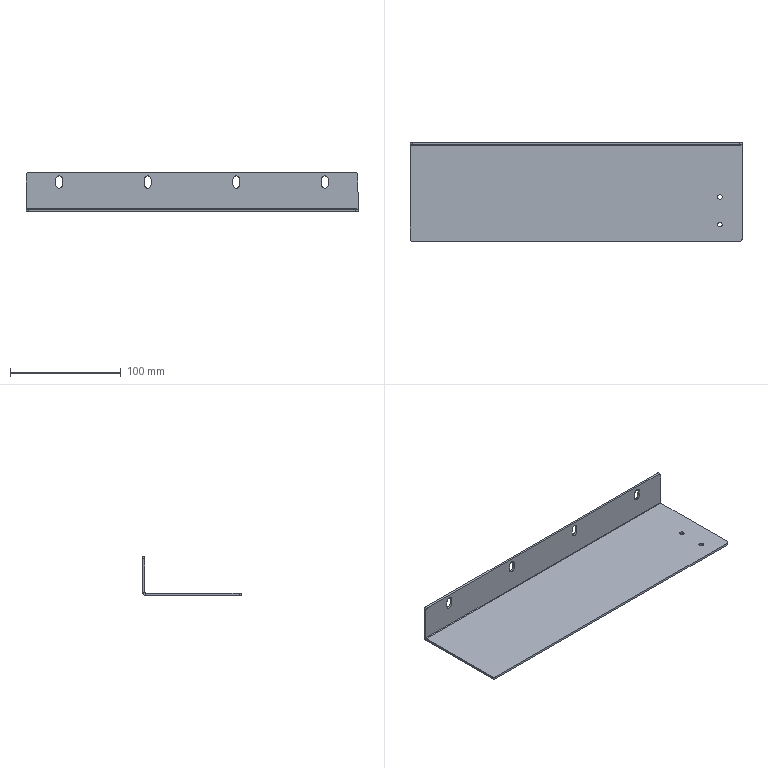Part | SolidWorks | features EdgeFlange 1, Fillet 1, FlatPattern 1, HoleWzd 1, ICE 1, LPattern 1, SMBaseFlange 1, SheetMetal 1 | 1 solid | 42 faces | box 300 x 89 x 35 mm | volume 72285 mm3 | cylinder 22 | plane 20 | commonest cylinder face diameters 6 x12 4 x4 4.2 x4 1 x1 5 x1
STEP:
#1=CARTESIAN_POINT('',(-37.,44.5,22.));
#2=VERTEX_POINT('',#1);
#3=CARTESIAN_POINT('',(-40.,44.5,19.));
#4=VERTEX_POINT('',#3);
#5=CARTESIAN_POINT('',(-40.,44.5,22.));
#6=DIRECTION('',(0.,1.,0.));
#7=DIRECTION('',(0.,0.,-1.));
#8=AXIS2_PLACEMENT_3D('',#5,#6,#7);
#9=CIRCLE('',#8,3.);
#10=EDGE_CURVE('',#2,#4,#9,.T.);
#11=ORIENTED_EDGE('',*,*,#10,.T.);
#12=CARTESIAN_POINT('',(-40.,42.5,19.));
#13=VERTEX_POINT('',#12);
#14=CARTESIAN_POINT('',(-40.,44.501,19.));
#15=DIRECTION('',(0.,-1.,0.));
#16=VECTOR('',#15,1000.);
#17=LINE('',#14,#16);
#18=EDGE_CURVE('',#4,#13,#17,.T.);
#19=ORIENTED_EDGE('',*,*,#18,.T.);
#20=CARTESIAN_POINT('',(-37.,42.5,22.));
#21=VERTEX_POINT('',#20);
#22=CARTESIAN_POINT('',(-40.,42.5,22.));
#23=DIRECTION('',(0.,-1.,0.));
#24=DIRECTION('',(0.,0.,-1.));
#25=AXIS2_PLACEMENT_3D('',#22,#23,#24);
#26=CIRCLE('',#25,3.);
#27=EDGE_CURVE('',#13,#21,#26,.T.);
#28=ORIENTED_EDGE('',*,*,#27,.T.);
#29=CARTESIAN_POINT('',(-37.,44.501,22.));
#30=DIRECTION('',(0.,-1.,0.));
#31=VECTOR('',#30,1000.);
#32=LINE('',#29,#31);
#33=EDGE_CURVE('',#2,#21,#32,.T.);
#34=ORIENTED_EDGE('',*,*,#33,.F.);
#35=EDGE_LOOP('',(#11,#19,#28,#34));
#36=FACE_OUTER_BOUND('',#35,.T.);
#37=CARTESIAN_POINT('',(-40.,44.501,22.));
#38=DIRECTION('',(0.,-1.,0.));
#39=DIRECTION('',(0.,0.,-1.));
#40=AXIS2_PLACEMENT_3D('',#37,#38,#39);
#41=CYLINDRICAL_SURFACE('',#40,3.);
#42=ADVANCED_FACE('',(#36),#41,.F.);
#43=CARTESIAN_POINT('',(-117.,44.5,22.));
#44=VERTEX_POINT('',#43);
#45=CARTESIAN_POINT('',(-120.,44.5,19.));
#46=VERTEX_POINT('',#45);
#47=CARTESIAN_POINT('',(-120.,44.5,22.));
#48=DIRECTION('',(0.,1.,0.));
#49=DIRECTION('',(0.,0.,-1.));
#50=AXIS2_PLACEMENT_3D('',#47,#48,#49);
#51=CIRCLE('',#50,3.);
#52=EDGE_CURVE('',#44,#46,#51,.T.);
#53=ORIENTED_EDGE('',*,*,#52,.T.);
#54=CARTESIAN_POINT('',(-120.,42.5,19.));
#55=VERTEX_POINT('',#54);
#56=CARTESIAN_POINT('',(-120.,44.501,19.));
#57=DIRECTION('',(0.,-1.,0.));
#58=VECTOR('',#57,1000.);
#59=LINE('',#56,#58);
#60=EDGE_CURVE('',#46,#55,#59,.T.);
#61=ORIENTED_EDGE('',*,*,#60,.T.);
#62=CARTESIAN_POINT('',(-117.,42.5,22.));
#63=VERTEX_POINT('',#62);
#64=CARTESIAN_POINT('',(-120.,42.5,22.));
#65=DIRECTION('',(0.,-1.,0.));
#66=DIRECTION('',(0.,0.,-1.));
#67=AXIS2_PLACEMENT_3D('',#64,#65,#66);
#68=CIRCLE('',#67,3.);
#69=EDGE_CURVE('',#55,#63,#68,.T.);
#70=ORIENTED_EDGE('',*,*,#69,.T.);
#71=CARTESIAN_POINT('',(-117.,44.501,22.));
#72=DIRECTION('',(0.,-1.,0.));
#73=VECTOR('',#72,1000.);
#74=LINE('',#71,#73);
#75=EDGE_CURVE('',#44,#63,#74,.T.);
#76=ORIENTED_EDGE('',*,*,#75,.F.);
#77=EDGE_LOOP('',(#53,#61,#70,#76));
#78=FACE_OUTER_BOUND('',#77,.T.);
#79=CARTESIAN_POINT('',(-120.,44.501,22.));
#80=DIRECTION('',(0.,-1.,0.));
#81=DIRECTION('',(0.,0.,-1.));
#82=AXIS2_PLACEMENT_3D('',#79,#80,#81);
#83=CYLINDRICAL_SURFACE('',#82,3.);
#84=ADVANCED_FACE('',(#78),#83,.F.);
#85=CARTESIAN_POINT('',(127.9,-29.5,-2.));
#86=VERTEX_POINT('',#85);
#87=CARTESIAN_POINT('',(132.1,-29.5,-2.));
#88=VERTEX_POINT('',#87);
#89=CARTESIAN_POINT('',(130.,-29.5,-2.));
#90=DIRECTION('',(0.,0.,1.));
#91=DIRECTION('',(1.,0.,0.));
#92=AXIS2_PLACEMENT_3D('',#89,#90,#91);
#93=CIRCLE('',#92,2.1);
#94=EDGE_CURVE('',#86,#88,#93,.T.);
#95=ORIENTED_EDGE('',*,*,#94,.F.);
#96=CARTESIAN_POINT('',(127.9,-29.5,0.));
#97=VERTEX_POINT('',#96);
#98=CARTESIAN_POINT('',(127.9,-29.5,0.));
#99=DIRECTION('',(0.,0.,1.));
#100=VECTOR('',#99,1000.);
#101=LINE('',#98,#100);
#102=EDGE_CURVE('',#86,#97,#101,.T.);
#103=ORIENTED_EDGE('',*,*,#102,.T.);
#104=CARTESIAN_POINT('',(132.1,-29.5,0.));
#105=VERTEX_POINT('',#104);
#106=CARTESIAN_POINT('',(130.,-29.5,0.));
#107=DIRECTION('',(0.,0.,1.));
#108=DIRECTION('',(1.,0.,0.));
#109=AXIS2_PLACEMENT_3D('',#106,#107,#108);
#110=CIRCLE('',#109,2.1);
#111=EDGE_CURVE('',#97,#105,#110,.T.);
#112=ORIENTED_EDGE('',*,*,#111,.T.);
#113=CARTESIAN_POINT('',(132.1,-29.5,0.));
#114=DIRECTION('',(0.,0.,1.));
#115=VECTOR('',#114,1000.);
#116=LINE('',#113,#115);
#117=EDGE_CURVE('',#88,#105,#116,.T.);
#118=ORIENTED_EDGE('',*,*,#117,.F.);
#119=EDGE_LOOP('',(#95,#103,#112,#118));
#120=FACE_OUTER_BOUND('',#119,.T.);
#121=CARTESIAN_POINT('',(130.,-29.5,0.));
#122=DIRECTION('',(0.,0.,1.));
#123=DIRECTION('',(1.,0.,0.));
#124=AXIS2_PLACEMENT_3D('',#121,#122,#123);
#125=CYLINDRICAL_SURFACE('',#124,2.1);
#126=ADVANCED_FACE('',(#120),#125,.F.);
#127=CARTESIAN_POINT('',(127.9,-4.5,-2.));
#128=VERTEX_POINT('',#127);
#129=CARTESIAN_POINT('',(132.1,-4.5,-2.));
#130=VERTEX_POINT('',#129);
#131=CARTESIAN_POINT('',(130.,-4.5,-2.));
#132=DIRECTION('',(0.,0.,1.));
#133=DIRECTION('',(1.,0.,0.));
#134=AXIS2_PLACEMENT_3D('',#131,#132,#133);
#135=CIRCLE('',#134,2.1);
#136=EDGE_CURVE('',#128,#130,#135,.T.);
#137=ORIENTED_EDGE('',*,*,#136,.F.);
#138=CARTESIAN_POINT('',(127.9,-4.5,0.));
#139=VERTEX_POINT('',#138);
#140=CARTESIAN_POINT('',(127.9,-4.5,0.));
#141=DIRECTION('',(0.,0.,1.));
#142=VECTOR('',#141,1000.);
#143=LINE('',#140,#142);
#144=EDGE_CURVE('',#128,#139,#143,.T.);
#145=ORIENTED_EDGE('',*,*,#144,.T.);
#146=CARTESIAN_POINT('',(132.1,-4.5,0.));
#147=VERTEX_POINT('',#146);
#148=CARTESIAN_POINT('',(130.,-4.5,0.));
#149=DIRECTION('',(0.,0.,1.));
#150=DIRECTION('',(1.,0.,0.));
#151=AXIS2_PLACEMENT_3D('',#148,#149,#150);
#152=CIRCLE('',#151,2.1);
#153=EDGE_CURVE('',#139,#147,#152,.T.);
#154=ORIENTED_EDGE('',*,*,#153,.T.);
#155=CARTESIAN_POINT('',(132.1,-4.5,0.));
#156=DIRECTION('',(0.,0.,1.));
#157=VECTOR('',#156,1000.);
#158=LINE('',#155,#157);
#159=EDGE_CURVE('',#130,#147,#158,.T.);
#160=ORIENTED_EDGE('',*,*,#159,.F.);
#161=EDGE_LOOP('',(#137,#145,#154,#160));
#162=FACE_OUTER_BOUND('',#161,.T.);
#163=CARTESIAN_POINT('',(130.,-4.5,0.));
#164=DIRECTION('',(0.,0.,1.));
#165=DIRECTION('',(1.,0.,0.));
#166=AXIS2_PLACEMENT_3D('',#163,#164,#165);
#167=CYLINDRICAL_SURFACE('',#166,2.1);
#168=ADVANCED_FACE('',(#162),#167,.F.);
#169=CARTESIAN_POINT('',(43.,44.5,22.));
#170=VERTEX_POINT('',#169);
#171=CARTESIAN_POINT('',(40.,44.5,19.));
#172=VERTEX_POINT('',#171);
#173=CARTESIAN_POINT('',(40.,44.5,22.));
#174=DIRECTION('',(0.,1.,0.));
#175=DIRECTION('',(0.,0.,-1.));
#176=AXIS2_PLACEMENT_3D('',#173,#174,#175);
#177=CIRCLE('',#176,3.);
#178=EDGE_CURVE('',#170,#172,#177,.T.);
#179=ORIENTED_EDGE('',*,*,#178,.T.);
#180=CARTESIAN_POINT('',(40.,42.5,19.));
#181=VERTEX_POINT('',#180);
#182=CARTESIAN_POINT('',(40.,44.501,19.));
#183=DIRECTION('',(0.,-1.,0.));
#184=VECTOR('',#183,1000.);
#185=LINE('',#182,#184);
#186=EDGE_CURVE('',#172,#181,#185,.T.);
#187=ORIENTED_EDGE('',*,*,#186,.T.);
#188=CARTESIAN_POINT('',(43.,42.5,22.));
#189=VERTEX_POINT('',#188);
#190=CARTESIAN_POINT('',(40.,42.5,22.));
#191=DIRECTION('',(0.,-1.,0.));
#192=DIRECTION('',(0.,0.,-1.));
#193=AXIS2_PLACEMENT_3D('',#190,#191,#192);
#194=CIRCLE('',#193,3.);
#195=EDGE_CURVE('',#181,#189,#194,.T.);
#196=ORIENTED_EDGE('',*,*,#195,.T.);
#197=CARTESIAN_POINT('',(43.,44.501,22.));
#198=DIRECTION('',(0.,-1.,0.));
#199=VECTOR('',#198,1000.);
#200=LINE('',#197,#199);
#201=EDGE_CURVE('',#170,#189,#200,.T.);
#202=ORIENTED_EDGE('',*,*,#201,.F.);
#203=EDGE_LOOP('',(#179,#187,#196,#202));
#204=FACE_OUTER_BOUND('',#203,.T.);
#205=CARTESIAN_POINT('',(40.,44.501,22.));
#206=DIRECTION('',(0.,-1.,0.));
#207=DIRECTION('',(0.,0.,-1.));
#208=AXIS2_PLACEMENT_3D('',#205,#206,#207);
#209=CYLINDRICAL_SURFACE('',#208,3.);
#210=ADVANCED_FACE('',(#204),#209,.F.);
#211=CARTESIAN_POINT('',(123.,44.5,22.));
#212=VERTEX_POINT('',#211);
#213=CARTESIAN_POINT('',(120.,44.5,19.));
#214=VERTEX_POINT('',#213);
#215=CARTESIAN_POINT('',(120.,44.5,22.));
#216=DIRECTION('',(0.,1.,0.));
#217=DIRECTION('',(0.,0.,-1.));
#218=AXIS2_PLACEMENT_3D('',#215,#216,#217);
#219=CIRCLE('',#218,3.);
#220=EDGE_CURVE('',#212,#214,#219,.T.);
#221=ORIENTED_EDGE('',*,*,#220,.T.);
#222=CARTESIAN_POINT('',(120.,42.5,19.));
#223=VERTEX_POINT('',#222);
#224=CARTESIAN_POINT('',(120.,44.501,19.));
#225=DIRECTION('',(0.,-1.,0.));
#226=VECTOR('',#225,1000.);
#227=LINE('',#224,#226);
#228=EDGE_CURVE('',#214,#223,#227,.T.);
#229=ORIENTED_EDGE('',*,*,#228,.T.);
#230=CARTESIAN_POINT('',(123.,42.5,22.));
#231=VERTEX_POINT('',#230);
#232=CARTESIAN_POINT('',(120.,42.5,22.));
#233=DIRECTION('',(0.,-1.,0.));
#234=DIRECTION('',(0.,0.,-1.));
#235=AXIS2_PLACEMENT_3D('',#232,#233,#234);
#236=CIRCLE('',#235,3.);
#237=EDGE_CURVE('',#223,#231,#236,.T.);
#238=ORIENTED_EDGE('',*,*,#237,.T.);
#239=CARTESIAN_POINT('',(123.,44.501,22.));
#240=DIRECTION('',(0.,-1.,0.));
#241=VECTOR('',#240,1000.);
#242=LINE('',#239,#241);
#243=EDGE_CURVE('',#212,#231,#242,.T.);
#244=ORIENTED_EDGE('',*,*,#243,.F.);
#245=EDGE_LOOP('',(#221,#229,#238,#244));
#246=FACE_OUTER_BOUND('',#245,.T.);
#247=CARTESIAN_POINT('',(120.,44.501,22.));
#248=DIRECTION('',(0.,-1.,0.));
#249=DIRECTION('',(0.,0.,-1.));
#250=AXIS2_PLACEMENT_3D('',#247,#248,#249);
#251=CYLINDRICAL_SURFACE('',#250,3.);
#252=ADVANCED_FACE('',(#246),#251,.F.);
#253=CARTESIAN_POINT('',(117.,44.5,22.));
#254=VERTEX_POINT('',#253);
#255=CARTESIAN_POINT('',(117.,44.5,27.));
#256=VERTEX_POINT('',#255);
#257=CARTESIAN_POINT('',(117.,44.5,27.));
#258=DIRECTION('',(0.,0.,1.));
#259=VECTOR('',#258,1000.);
#260=LINE('',#257,#259);
#261=EDGE_CURVE('',#254,#256,#260,.T.);
#262=ORIENTED_EDGE('',*,*,#261,.T.);
#263=CARTESIAN_POINT('',(117.,42.5,27.));
#264=VERTEX_POINT('',#263);
#265=CARTESIAN_POINT('',(117.,44.501,27.));
#266=DIRECTION('',(0.,-1.,0.));
#267=VECTOR('',#266,1000.);
#268=LINE('',#265,#267);
#269=EDGE_CURVE('',#256,#264,#268,.T.);
#270=ORIENTED_EDGE('',*,*,#269,.T.);
#271=CARTESIAN_POINT('',(117.,42.5,22.));
#272=VERTEX_POINT('',#271);
#273=CARTESIAN_POINT('',(117.,42.5,27.));
#274=DIRECTION('',(0.,0.,-1.));
#275=VECTOR('',#274,1000.);
#276=LINE('',#273,#275);
#277=EDGE_CURVE('',#264,#272,#276,.T.);
#278=ORIENTED_EDGE('',*,*,#277,.T.);
#279=CARTESIAN_POINT('',(117.,44.501,22.));
#280=DIRECTION('',(0.,-1.,0.));
#281=VECTOR('',#280,1000.);
#282=LINE('',#279,#281);
#283=EDGE_CURVE('',#254,#272,#282,.T.);
#284=ORIENTED_EDGE('',*,*,#283,.F.);
#285=EDGE_LOOP('',(#262,#270,#278,#284));
#286=FACE_OUTER_BOUND('',#285,.T.);
#287=CARTESIAN_POINT('',(117.,44.501,27.));
#288=DIRECTION('',(-1.,0.,0.));
#289=DIRECTION('',(0.,-1.,0.));
#290=AXIS2_PLACEMENT_3D('',#287,#288,#289);
#291=PLANE('',#290);
#292=ADVANCED_FACE('',(#286),#291,.F.);
#293=ORIENTED_EDGE('',*,*,#228,.F.);
#294=CARTESIAN_POINT('',(120.,44.5,22.));
#295=DIRECTION('',(0.,1.,0.));
#296=DIRECTION('',(0.,0.,-1.));
#297=AXIS2_PLACEMENT_3D('',#294,#295,#296);
#298=CIRCLE('',#297,3.);
#299=EDGE_CURVE('',#214,#254,#298,.T.);
#300=ORIENTED_EDGE('',*,*,#299,.T.);
#301=ORIENTED_EDGE('',*,*,#283,.T.);
#302=CARTESIAN_POINT('',(120.,42.5,22.));
#303=DIRECTION('',(0.,-1.,0.));
#304=DIRECTION('',(0.,0.,-1.));
#305=AXIS2_PLACEMENT_3D('',#302,#303,#304);
#306=CIRCLE('',#305,3.);
#307=EDGE_CURVE('',#272,#223,#306,.T.);
#308=ORIENTED_EDGE('',*,*,#307,.T.);
#309=EDGE_LOOP('',(#293,#300,#301,#308));
#310=FACE_OUTER_BOUND('',#309,.T.);
#311=CARTESIAN_POINT('',(120.,44.501,22.));
#312=DIRECTION('',(0.,-1.,0.));
#313=DIRECTION('',(0.,0.,-1.));
#314=AXIS2_PLACEMENT_3D('',#311,#312,#313);
#315=CYLINDRICAL_SURFACE('',#314,3.);
#316=ADVANCED_FACE('',(#310),#315,.F.);
#317=CARTESIAN_POINT('',(123.,44.5,27.));
#318=VERTEX_POINT('',#317);
#319=CARTESIAN_POINT('',(123.,44.5,27.));
#320=DIRECTION('',(0.,0.,-1.));
#321=VECTOR('',#320,1000.);
#322=LINE('',#319,#321);
#323=EDGE_CURVE('',#318,#212,#322,.T.);
#324=ORIENTED_EDGE('',*,*,#323,.T.);
#325=ORIENTED_EDGE('',*,*,#243,.T.);
#326=CARTESIAN_POINT('',(123.,42.5,27.));
#327=VERTEX_POINT('',#326);
#328=CARTESIAN_POINT('',(123.,42.5,27.));
#329=DIRECTION('',(0.,0.,1.));
#330=VECTOR('',#329,1000.);
#331=LINE('',#328,#330);
#332=EDGE_CURVE('',#231,#327,#331,.T.);
#333=ORIENTED_EDGE('',*,*,#332,.T.);
#334=CARTESIAN_POINT('',(123.,44.501,27.));
#335=DIRECTION('',(0.,-1.,0.));
#336=VECTOR('',#335,1000.);
#337=LINE('',#334,#336);
#338=EDGE_CURVE('',#318,#327,#337,.T.);
#339=ORIENTED_EDGE('',*,*,#338,.F.);
#340=EDGE_LOOP('',(#324,#325,#333,#339));
#341=FACE_OUTER_BOUND('',#340,.T.);
#342=CARTESIAN_POINT('',(123.,44.501,27.));
#343=DIRECTION('',(1.,0.,0.));
#344=DIRECTION('',(0.,1.,0.));
#345=AXIS2_PLACEMENT_3D('',#342,#343,#344);
#346=PLANE('',#345);
#347=ADVANCED_FACE('',(#341),#346,.F.);
#348=CARTESIAN_POINT('',(120.,44.5,27.));
#349=DIRECTION('',(0.,1.,0.));
#350=DIRECTION('',(0.,0.,-1.));
#351=AXIS2_PLACEMENT_3D('',#348,#349,#350);
#352=CIRCLE('',#351,3.);
#353=EDGE_CURVE('',#256,#318,#352,.T.);
#354=ORIENTED_EDGE('',*,*,#353,.T.);
#355=ORIENTED_EDGE('',*,*,#338,.T.);
#356=CARTESIAN_POINT('',(120.,42.5,27.));
#357=DIRECTION('',(0.,-1.,0.));
#358=DIRECTION('',(0.,0.,-1.));
#359=AXIS2_PLACEMENT_3D('',#356,#357,#358);
#360=CIRCLE('',#359,3.);
#361=EDGE_CURVE('',#327,#264,#360,.T.);
#362=ORIENTED_EDGE('',*,*,#361,.T.);
#363=ORIENTED_EDGE('',*,*,#269,.F.);
#364=EDGE_LOOP('',(#354,#355,#362,#363));
#365=FACE_OUTER_BOUND('',#364,.T.);
#366=CARTESIAN_POINT('',(120.,44.501,27.));
#367=DIRECTION('',(0.,-1.,0.));
#368=DIRECTION('',(0.,0.,-1.));
#369=AXIS2_PLACEMENT_3D('',#366,#367,#368);
#370=CYLINDRICAL_SURFACE('',#369,3.);
#371=ADVANCED_FACE('',(#365),#370,.F.);
#372=CARTESIAN_POINT('',(37.,44.5,22.));
#373=VERTEX_POINT('',#372);
#374=CARTESIAN_POINT('',(37.,44.5,27.));
#375=VERTEX_POINT('',#374);
#376=CARTESIAN_POINT('',(37.,44.5,27.));
#377=DIRECTION('',(0.,0.,1.));
#378=VECTOR('',#377,1000.);
#379=LINE('',#376,#378);
#380=EDGE_CURVE('',#373,#375,#379,.T.);
#381=ORIENTED_EDGE('',*,*,#380,.T.);
#382=CARTESIAN_POINT('',(37.,42.5,27.));
#383=VERTEX_POINT('',#382);
#384=CARTESIAN_POINT('',(37.,44.501,27.));
#385=DIRECTION('',(0.,-1.,0.));
#386=VECTOR('',#385,1000.);
#387=LINE('',#384,#386);
#388=EDGE_CURVE('',#375,#383,#387,.T.);
#389=ORIENTED_EDGE('',*,*,#388,.T.);
#390=CARTESIAN_POINT('',(37.,42.5,22.));
#391=VERTEX_POINT('',#390);
#392=CARTESIAN_POINT('',(37.,42.5,27.));
#393=DIRECTION('',(0.,0.,-1.));
#394=VECTOR('',#393,1000.);
#395=LINE('',#392,#394);
#396=EDGE_CURVE('',#383,#391,#395,.T.);
#397=ORIENTED_EDGE('',*,*,#396,.T.);
#398=CARTESIAN_POINT('',(37.,44.501,22.));
#399=DIRECTION('',(0.,-1.,0.));
#400=VECTOR('',#399,1000.);
#401=LINE('',#398,#400);
#402=EDGE_CURVE('',#373,#391,#401,.T.);
#403=ORIENTED_EDGE('',*,*,#402,.F.);
#404=EDGE_LOOP('',(#381,#389,#397,#403));
#405=FACE_OUTER_BOUND('',#404,.T.);
#406=CARTESIAN_POINT('',(37.,44.501,27.));
#407=DIRECTION('',(-1.,0.,0.));
#408=DIRECTION('',(0.,-1.,0.));
#409=AXIS2_PLACEMENT_3D('',#406,#407,#408);
#410=PLANE('',#409);
#411=ADVANCED_FACE('',(#405),#410,.F.);
#412=ORIENTED_EDGE('',*,*,#186,.F.);
#413=CARTESIAN_POINT('',(40.,44.5,22.));
#414=DIRECTION('',(0.,1.,0.));
#415=DIRECTION('',(0.,0.,-1.));
#416=AXIS2_PLACEMENT_3D('',#413,#414,#415);
#417=CIRCLE('',#416,3.);
#418=EDGE_CURVE('',#172,#373,#417,.T.);
#419=ORIENTED_EDGE('',*,*,#418,.T.);
#420=ORIENTED_EDGE('',*,*,#402,.T.);
#421=CARTESIAN_POINT('',(40.,42.5,22.));
#422=DIRECTION('',(0.,-1.,0.));
#423=DIRECTION('',(0.,0.,-1.));
#424=AXIS2_PLACEMENT_3D('',#421,#422,#423);
#425=CIRCLE('',#424,3.);
#426=EDGE_CURVE('',#391,#181,#425,.T.);
#427=ORIENTED_EDGE('',*,*,#426,.T.);
#428=EDGE_LOOP('',(#412,#419,#420,#427));
#429=FACE_OUTER_BOUND('',#428,.T.);
#430=CARTESIAN_POINT('',(40.,44.501,22.));
#431=DIRECTION('',(0.,-1.,0.));
#432=DIRECTION('',(0.,0.,-1.));
#433=AXIS2_PLACEMENT_3D('',#430,#431,#432);
#434=CYLINDRICAL_SURFACE('',#433,3.);
#435=ADVANCED_FACE('',(#429),#434,.F.);
#436=CARTESIAN_POINT('',(43.,44.5,27.));
#437=VERTEX_POINT('',#436);
#438=CARTESIAN_POINT('',(43.,44.5,27.));
#439=DIRECTION('',(0.,0.,-1.));
#440=VECTOR('',#439,1000.);
#441=LINE('',#438,#440);
#442=EDGE_CURVE('',#437,#170,#441,.T.);
#443=ORIENTED_EDGE('',*,*,#442,.T.);
#444=ORIENTED_EDGE('',*,*,#201,.T.);
#445=CARTESIAN_POINT('',(43.,42.5,27.));
#446=VERTEX_POINT('',#445);
#447=CARTESIAN_POINT('',(43.,42.5,27.));
#448=DIRECTION('',(0.,0.,1.));
#449=VECTOR('',#448,1000.);
#450=LINE('',#447,#449);
#451=EDGE_CURVE('',#189,#446,#450,.T.);
#452=ORIENTED_EDGE('',*,*,#451,.T.);
#453=CARTESIAN_POINT('',(43.,44.501,27.));
#454=DIRECTION('',(0.,-1.,0.));
#455=VECTOR('',#454,1000.);
#456=LINE('',#453,#455);
#457=EDGE_CURVE('',#437,#446,#456,.T.);
#458=ORIENTED_EDGE('',*,*,#457,.F.);
#459=EDGE_LOOP('',(#443,#444,#452,#458));
#460=FACE_OUTER_BOUND('',#459,.T.);
#461=CARTESIAN_POINT('',(43.,44.501,27.));
#462=DIRECTION('',(1.,0.,0.));
#463=DIRECTION('',(0.,1.,0.));
#464=AXIS2_PLACEMENT_3D('',#461,#462,#463);
#465=PLANE('',#464);
#466=ADVANCED_FACE('',(#460),#465,.F.);
#467=CARTESIAN_POINT('',(40.,44.5,27.));
#468=DIRECTION('',(0.,1.,0.));
#469=DIRECTION('',(0.,0.,-1.));
#470=AXIS2_PLACEMENT_3D('',#467,#468,#469);
#471=CIRCLE('',#470,3.);
#472=EDGE_CURVE('',#375,#437,#471,.T.);
#473=ORIENTED_EDGE('',*,*,#472,.T.);
#474=ORIENTED_EDGE('',*,*,#457,.T.);
#475=CARTESIAN_POINT('',(40.,42.5,27.));
#476=DIRECTION('',(0.,-1.,0.));
#477=DIRECTION('',(0.,0.,-1.));
#478=AXIS2_PLACEMENT_3D('',#475,#476,#477);
#479=CIRCLE('',#478,3.);
#480=EDGE_CURVE('',#446,#383,#479,.T.);
#481=ORIENTED_EDGE('',*,*,#480,.T.);
#482=ORIENTED_EDGE('',*,*,#388,.F.);
#483=EDGE_LOOP('',(#473,#474,#481,#482));
#484=FACE_OUTER_BOUND('',#483,.T.);
#485=CARTESIAN_POINT('',(40.,44.501,27.));
#486=DIRECTION('',(0.,-1.,0.));
#487=DIRECTION('',(0.,0.,-1.));
#488=AXIS2_PLACEMENT_3D('',#485,#486,#487);
#489=CYLINDRICAL_SURFACE('',#488,3.);
#490=ADVANCED_FACE('',(#484),#489,.F.);
#491=CARTESIAN_POINT('',(-150.,42.,-2.));
#492=VERTEX_POINT('',#491);
#493=CARTESIAN_POINT('',(-150.,-42.5,-2.));
#494=VERTEX_POINT('',#493);
#495=CARTESIAN_POINT('',(-150.,-44.5,-2.));
#496=DIRECTION('',(0.,-1.,0.));
#497=VECTOR('',#496,1000.);
#498=LINE('',#495,#497);
#499=EDGE_CURVE('',#492,#494,#498,.T.);
#500=ORIENTED_EDGE('',*,*,#499,.T.);
#501=CARTESIAN_POINT('',(-150.,-42.5,0.));
#502=VERTEX_POINT('',#501);
#503=CARTESIAN_POINT('',(-150.,-42.5,-2.));
#504=DIRECTION('',(0.,0.,1.));
#505=VECTOR('',#504,1000.);
#506=LINE('',#503,#505);
#507=EDGE_CURVE('',#494,#502,#506,.T.);
#508=ORIENTED_EDGE('',*,*,#507,.T.);
#509=CARTESIAN_POINT('',(-150.,42.,0.));
#510=VERTEX_POINT('',#509);
#511=CARTESIAN_POINT('',(-150.,-44.5,0.));
#512=DIRECTION('',(0.,-1.,0.));
#513=VECTOR('',#512,1000.);
#514=LINE('',#511,#513);
#515=EDGE_CURVE('',#510,#502,#514,.T.);
#516=ORIENTED_EDGE('',*,*,#515,.F.);
#517=CARTESIAN_POINT('',(-150.,42.,0.));
#518=DIRECTION('',(0.,0.,-1.));
#519=VECTOR('',#518,1000.);
#520=LINE('',#517,#519);
#521=EDGE_CURVE('',#510,#492,#520,.T.);
#522=ORIENTED_EDGE('',*,*,#521,.T.);
#523=EDGE_LOOP('',(#500,#508,#516,#522));
#524=FACE_OUTER_BOUND('',#523,.T.);
#525=CARTESIAN_POINT('',(-150.,-44.5,-2.));
#526=DIRECTION('',(-1.,0.,0.));
#527=DIRECTION('',(0.,0.,1.));
#528=AXIS2_PLACEMENT_3D('',#525,#526,#527);
#529=PLANE('',#528);
#530=ADVANCED_FACE('',(#524),#529,.T.);
#531=CARTESIAN_POINT('',(130.,-29.5,-2.));
#532=DIRECTION('',(0.,0.,1.));
#533=DIRECTION('',(1.,0.,0.));
#534=AXIS2_PLACEMENT_3D('',#531,#532,#533);
#535=CIRCLE('',#534,2.1);
#536=EDGE_CURVE('',#88,#86,#535,.T.);
#537=ORIENTED_EDGE('',*,*,#536,.T.);
#538=ORIENTED_EDGE('',*,*,#94,.T.);
#539=EDGE_LOOP('',(#537,#538));
#540=FACE_BOUND('',#539,.T.);
#541=CARTESIAN_POINT('',(130.,-4.5,-2.));
#542=DIRECTION('',(0.,0.,1.));
#543=DIRECTION('',(1.,0.,0.));
#544=AXIS2_PLACEMENT_3D('',#541,#542,#543);
#545=CIRCLE('',#544,2.1);
#546=EDGE_CURVE('',#130,#128,#545,.T.);
#547=ORIENTED_EDGE('',*,*,#546,.T.);
#548=ORIENTED_EDGE('',*,*,#136,.T.);
#549=EDGE_LOOP('',(#547,#548));
#550=FACE_BOUND('',#549,.T.);
#551=CARTESIAN_POINT('',(-148.,-44.5,-2.));
#552=VERTEX_POINT('',#551);
#553=CARTESIAN_POINT('',(148.,-44.5,-2.));
#554=VERTEX_POINT('',#553);
#555=CARTESIAN_POINT('',(150.,-44.5,-2.));
#556=DIRECTION('',(1.,0.,0.));
#557=VECTOR('',#556,1000.);
#558=LINE('',#555,#557);
#559=EDGE_CURVE('',#552,#554,#558,.T.);
#560=ORIENTED_EDGE('',*,*,#559,.F.);
#561=CARTESIAN_POINT('',(-148.,-42.5,-2.));
#562=DIRECTION('',(0.,0.,-1.));
#563=DIRECTION('',(1.,0.,0.));
#564=AXIS2_PLACEMENT_3D('',#561,#562,#563);
#565=CIRCLE('',#564,2.);
#566=EDGE_CURVE('',#552,#494,#565,.T.);
#567=ORIENTED_EDGE('',*,*,#566,.T.);
#568=ORIENTED_EDGE('',*,*,#499,.F.);
#569=CARTESIAN_POINT('',(150.,42.,-2.));
#570=VERTEX_POINT('',#569);
#571=CARTESIAN_POINT('',(-150.,42.,-2.));
#572=DIRECTION('',(1.,0.,0.));
#573=VECTOR('',#572,1000.);
#574=LINE('',#571,#573);
#575=EDGE_CURVE('',#492,#570,#574,.T.);
#576=ORIENTED_EDGE('',*,*,#575,.T.);
#577=CARTESIAN_POINT('',(150.,-42.5,-2.));
#578=VERTEX_POINT('',#577);
#579=CARTESIAN_POINT('',(150.,-44.5,-2.));
#580=DIRECTION('',(0.,1.,0.));
#581=VECTOR('',#580,1000.);
#582=LINE('',#579,#581);
#583=EDGE_CURVE('',#578,#570,#582,.T.);
#584=ORIENTED_EDGE('',*,*,#583,.F.);
#585=CARTESIAN_POINT('',(148.,-42.5,-2.));
#586=DIRECTION('',(0.,0.,-1.));
#587=DIRECTION('',(1.,0.,0.));
#588=AXIS2_PLACEMENT_3D('',#585,#586,#587);
#589=CIRCLE('',#588,2.);
#590=EDGE_CURVE('',#578,#554,#589,.T.);
#591=ORIENTED_EDGE('',*,*,#590,.T.);
#592=EDGE_LOOP('',(#560,#567,#568,#576,#584,#591));
#593=FACE_OUTER_BOUND('',#592,.T.);
#594=CARTESIAN_POINT('',(0.,0.,-2.));
#595=DIRECTION('',(0.,0.,1.));
#596=DIRECTION('',(1.,0.,0.));
#597=AXIS2_PLACEMENT_3D('',#594,#595,#596);
#598=PLANE('',#597);
#599=ADVANCED_FACE('',(#540,#550,#593),#598,.F.);
#600=CARTESIAN_POINT('',(130.,-29.5,0.));
#601=DIRECTION('',(0.,0.,1.));
#602=DIRECTION('',(1.,0.,0.));
#603=AXIS2_PLACEMENT_3D('',#600,#601,#602);
#604=CIRCLE('',#603,2.1);
#605=EDGE_CURVE('',#105,#97,#604,.T.);
#606=ORIENTED_EDGE('',*,*,#605,.F.);
#607=ORIENTED_EDGE('',*,*,#111,.F.);
#608=EDGE_LOOP('',(#606,#607));
#609=FACE_BOUND('',#608,.T.);
#610=CARTESIAN_POINT('',(130.,-4.5,0.));
#611=DIRECTION('',(0.,0.,1.));
#612=DIRECTION('',(1.,0.,0.));
#613=AXIS2_PLACEMENT_3D('',#610,#611,#612);
#614=CIRCLE('',#613,2.1);
#615=EDGE_CURVE('',#147,#139,#614,.T.);
#616=ORIENTED_EDGE('',*,*,#615,.F.);
#617=ORIENTED_EDGE('',*,*,#153,.F.);
#618=EDGE_LOOP('',(#616,#617));
#619=FACE_BOUND('',#618,.T.);
#620=ORIENTED_EDGE('',*,*,#515,.T.);
#621=CARTESIAN_POINT('',(-148.,-44.5,0.));
#622=VERTEX_POINT('',#621);
#623=CARTESIAN_POINT('',(-148.,-42.5,0.));
#624=DIRECTION('',(0.,0.,1.));
#625=DIRECTION('',(1.,0.,0.));
#626=AXIS2_PLACEMENT_3D('',#623,#624,#625);
#627=CIRCLE('',#626,2.);
#628=EDGE_CURVE('',#502,#622,#627,.T.);
#629=ORIENTED_EDGE('',*,*,#628,.T.);
#630=CARTESIAN_POINT('',(148.,-44.5,0.));
#631=VERTEX_POINT('',#630);
#632=CARTESIAN_POINT('',(150.,-44.5,0.));
#633=DIRECTION('',(1.,0.,0.));
#634=VECTOR('',#633,1000.);
#635=LINE('',#632,#634);
#636=EDGE_CURVE('',#622,#631,#635,.T.);
#637=ORIENTED_EDGE('',*,*,#636,.T.);
#638=CARTESIAN_POINT('',(150.,-42.5,0.));
#639=VERTEX_POINT('',#638);
#640=CARTESIAN_POINT('',(148.,-42.5,0.));
#641=DIRECTION('',(0.,0.,1.));
#642=DIRECTION('',(1.,0.,0.));
#643=AXIS2_PLACEMENT_3D('',#640,#641,#642);
#644=CIRCLE('',#643,2.);
#645=EDGE_CURVE('',#631,#639,#644,.T.);
#646=ORIENTED_EDGE('',*,*,#645,.T.);
#647=CARTESIAN_POINT('',(150.,42.,0.));
#648=VERTEX_POINT('',#647);
#649=CARTESIAN_POINT('',(150.,-44.5,0.));
#650=DIRECTION('',(0.,1.,0.));
#651=VECTOR('',#650,1000.);
#652=LINE('',#649,#651);
#653=EDGE_CURVE('',#639,#648,#652,.T.);
#654=ORIENTED_EDGE('',*,*,#653,.T.);
#655=CARTESIAN_POINT('',(-150.,42.,0.));
#656=DIRECTION('',(1.,0.,0.));
#657=VECTOR('',#656,1000.);
#658=LINE('',#655,#657);
#659=EDGE_CURVE('',#510,#648,#658,.T.);
#660=ORIENTED_EDGE('',*,*,#659,.F.);
#661=EDGE_LOOP('',(#620,#629,#637,#646,#654,#660));
#662=FACE_OUTER_BOUND('',#661,.T.);
#663=CARTESIAN_POINT('',(0.,0.,0.));
#664=DIRECTION('',(0.,0.,1.));
#665=DIRECTION('',(1.,0.,0.));
#666=AXIS2_PLACEMENT_3D('',#663,#664,#665);
#667=PLANE('',#666);
#668=ADVANCED_FACE('',(#609,#619,#662),#667,.T.);
#669=ORIENTED_EDGE('',*,*,#653,.F.);
#670=CARTESIAN_POINT('',(150.,-42.5,-2.));
#671=DIRECTION('',(0.,0.,-1.));
#672=VECTOR('',#671,1000.);
#673=LINE('',#670,#672);
#674=EDGE_CURVE('',#639,#578,#673,.T.);
#675=ORIENTED_EDGE('',*,*,#674,.T.);
#676=ORIENTED_EDGE('',*,*,#583,.T.);
#677=CARTESIAN_POINT('',(150.,42.,0.));
#678=DIRECTION('',(0.,0.,-1.));
#679=VECTOR('',#678,1000.);
#680=LINE('',#677,#679);
#681=EDGE_CURVE('',#648,#570,#680,.T.);
#682=ORIENTED_EDGE('',*,*,#681,.F.);
#683=EDGE_LOOP('',(#669,#675,#676,#682));
#684=FACE_OUTER_BOUND('',#683,.T.);
#685=CARTESIAN_POINT('',(150.,-44.5,-2.));
#686=DIRECTION('',(1.,0.,0.));
#687=DIRECTION('',(0.,0.,-1.));
#688=AXIS2_PLACEMENT_3D('',#685,#686,#687);
#689=PLANE('',#688);
#690=ADVANCED_FACE('',(#684),#689,.T.);
#691=ORIENTED_EDGE('',*,*,#636,.F.);
#692=CARTESIAN_POINT('',(-148.,-44.5,-2.));
#693=DIRECTION('',(0.,0.,-1.));
#694=VECTOR('',#693,1000.);
#695=LINE('',#692,#694);
#696=EDGE_CURVE('',#622,#552,#695,.T.);
#697=ORIENTED_EDGE('',*,*,#696,.T.);
#698=ORIENTED_EDGE('',*,*,#559,.T.);
#699=CARTESIAN_POINT('',(148.,-44.5,-2.));
#700=DIRECTION('',(0.,0.,1.));
#701=VECTOR('',#700,1000.);
#702=LINE('',#699,#701);
#703=EDGE_CURVE('',#554,#631,#702,.T.);
#704=ORIENTED_EDGE('',*,*,#703,.T.);
#705=EDGE_LOOP('',(#691,#697,#698,#704));
#706=FACE_OUTER_BOUND('',#705,.T.);
#707=CARTESIAN_POINT('',(150.,-44.5,-2.));
#708=DIRECTION('',(0.,-1.,0.));
#709=DIRECTION('',(1.,0.,0.));
#710=AXIS2_PLACEMENT_3D('',#707,#708,#709);
#711=PLANE('',#710);
#712=ADVANCED_FACE('',(#706),#711,.T.);
#713=CARTESIAN_POINT('',(150.,42.5,0.5));
#714=VERTEX_POINT('',#713);
#715=CARTESIAN_POINT('',(150.,44.5,0.5));
#716=VERTEX_POINT('',#715);
#717=CARTESIAN_POINT('',(150.,44.5,0.5));
#718=DIRECTION('',(0.,1.,0.));
#719=VECTOR('',#718,1000.);
#720=LINE('',#717,#719);
#721=EDGE_CURVE('',#714,#716,#720,.T.);
#722=ORIENTED_EDGE('',*,*,#721,.F.);
#723=CARTESIAN_POINT('',(150.,42.,0.5));
#724=DIRECTION('',(1.,0.,0.));
#725=DIRECTION('',(0.,0.,1.));
#726=AXIS2_PLACEMENT_3D('',#723,#724,#725);
#727=CIRCLE('',#726,0.5);
#728=EDGE_CURVE('',#648,#714,#727,.T.);
#729=ORIENTED_EDGE('',*,*,#728,.F.);
#730=ORIENTED_EDGE('',*,*,#681,.T.);
#731=CARTESIAN_POINT('',(150.,42.,0.5));
#732=DIRECTION('',(1.,0.,0.));
#733=DIRECTION('',(0.,0.,1.));
#734=AXIS2_PLACEMENT_3D('',#731,#732,#733);
#735=CIRCLE('',#734,2.5);
#736=EDGE_CURVE('',#570,#716,#735,.T.);
#737=ORIENTED_EDGE('',*,*,#736,.T.);
#738=EDGE_LOOP('',(#722,#729,#730,#737));
#739=FACE_OUTER_BOUND('',#738,.T.);
#740=CARTESIAN_POINT('',(150.,42.,0.5));
#741=DIRECTION('',(1.,0.,0.));
#742=DIRECTION('',(0.,0.,-1.));
#743=AXIS2_PLACEMENT_3D('',#740,#741,#742);
#744=PLANE('',#743);
#745=ADVANCED_FACE('',(#739),#744,.T.);
#746=CARTESIAN_POINT('',(-150.,42.5,0.5));
#747=VERTEX_POINT('',#746);
#748=CARTESIAN_POINT('',(-150.,42.,0.5));
#749=DIRECTION('',(-1.,0.,0.));
#750=DIRECTION('',(0.,0.,1.));
#751=AXIS2_PLACEMENT_3D('',#748,#749,#750);
#752=CIRCLE('',#751,0.5);
#753=EDGE_CURVE('',#747,#510,#752,.T.);
#754=ORIENTED_EDGE('',*,*,#753,.F.);
#755=CARTESIAN_POINT('',(-150.,44.5,0.5));
#756=VERTEX_POINT('',#755);
#757=CARTESIAN_POINT('',(-150.,42.5,0.5));
#758=DIRECTION('',(0.,1.,0.));
#759=VECTOR('',#758,1000.);
#760=LINE('',#757,#759);
#761=EDGE_CURVE('',#747,#756,#760,.T.);
#762=ORIENTED_EDGE('',*,*,#761,.T.);
#763=CARTESIAN_POINT('',(-150.,42.,0.5));
#764=DIRECTION('',(-1.,0.,0.));
#765=DIRECTION('',(0.,0.,1.));
#766=AXIS2_PLACEMENT_3D('',#763,#764,#765);
#767=CIRCLE('',#766,2.5);
#768=EDGE_CURVE('',#756,#492,#767,.T.);
#769=ORIENTED_EDGE('',*,*,#768,.T.);
#770=ORIENTED_EDGE('',*,*,#521,.F.);
#771=EDGE_LOOP('',(#754,#762,#769,#770));
#772=FACE_OUTER_BOUND('',#771,.T.);
#773=CARTESIAN_POINT('',(-150.,42.,0.5));
#774=DIRECTION('',(1.,0.,0.));
#775=DIRECTION('',(0.,0.,-1.));
#776=AXIS2_PLACEMENT_3D('',#773,#774,#775);
#777=PLANE('',#776);
#778=ADVANCED_FACE('',(#772),#777,.F.);
#779=ORIENTED_EDGE('',*,*,#575,.F.);
#780=ORIENTED_EDGE('',*,*,#768,.F.);
#781=CARTESIAN_POINT('',(150.,44.5,0.5));
#782=DIRECTION('',(1.,0.,0.));
#783=VECTOR('',#782,1000.);
#784=LINE('',#781,#783);
#785=EDGE_CURVE('',#756,#716,#784,.T.);
#786=ORIENTED_EDGE('',*,*,#785,.T.);
#787=ORIENTED_EDGE('',*,*,#736,.F.);
#788=EDGE_LOOP('',(#779,#780,#786,#787));
#789=FACE_OUTER_BOUND('',#788,.T.);
#790=CARTESIAN_POINT('',(-150.,42.,0.5));
#791=DIRECTION('',(-1.,0.,0.));
#792=DIRECTION('',(0.,1.,0.));
#793=AXIS2_PLACEMENT_3D('',#790,#791,#792);
#794=CYLINDRICAL_SURFACE('',#793,2.5);
#795=ADVANCED_FACE('',(#789),#794,.T.);
#796=ORIENTED_EDGE('',*,*,#659,.T.);
#797=ORIENTED_EDGE('',*,*,#728,.T.);
#798=CARTESIAN_POINT('',(150.,42.5,0.5));
#799=DIRECTION('',(-1.,0.,0.));
#800=VECTOR('',#799,1000.);
#801=LINE('',#798,#800);
#802=EDGE_CURVE('',#714,#747,#801,.T.);
#803=ORIENTED_EDGE('',*,*,#802,.T.);
#804=ORIENTED_EDGE('',*,*,#753,.T.);
#805=EDGE_LOOP('',(#796,#797,#803,#804));
#806=FACE_OUTER_BOUND('',#805,.T.);
#807=CARTESIAN_POINT('',(-150.,42.,0.5));
#808=DIRECTION('',(-1.,0.,0.));
#809=DIRECTION('',(0.,1.,0.));
#810=AXIS2_PLACEMENT_3D('',#807,#808,#809);
#811=CYLINDRICAL_SURFACE('',#810,0.5);
#812=ADVANCED_FACE('',(#806),#811,.F.);
#813=CARTESIAN_POINT('',(150.,44.5,31.));
#814=VERTEX_POINT('',#813);
#815=CARTESIAN_POINT('',(150.,44.5,0.));
#816=DIRECTION('',(0.,0.,-1.));
#817=VECTOR('',#816,1000.);
#818=LINE('',#815,#817);
#819=EDGE_CURVE('',#814,#716,#818,.T.);
#820=ORIENTED_EDGE('',*,*,#819,.F.);
#821=CARTESIAN_POINT('',(150.,42.5,31.));
#822=VERTEX_POINT('',#821);
#823=CARTESIAN_POINT('',(150.,44.5,31.));
#824=DIRECTION('',(0.,-1.,0.));
#825=VECTOR('',#824,1000.);
#826=LINE('',#823,#825);
#827=EDGE_CURVE('',#814,#822,#826,.T.);
#828=ORIENTED_EDGE('',*,*,#827,.T.);
#829=CARTESIAN_POINT('',(150.,42.5,0.));
#830=DIRECTION('',(0.,0.,-1.));
#831=VECTOR('',#830,1000.);
#832=LINE('',#829,#831);
#833=EDGE_CURVE('',#822,#714,#832,.T.);
#834=ORIENTED_EDGE('',*,*,#833,.T.);
#835=ORIENTED_EDGE('',*,*,#721,.T.);
#836=EDGE_LOOP('',(#820,#828,#834,#835));
#837=FACE_OUTER_BOUND('',#836,.T.);
#838=CARTESIAN_POINT('',(150.,44.5,0.));
#839=DIRECTION('',(-1.,0.,0.));
#840=DIRECTION('',(0.,0.,1.));
#841=AXIS2_PLACEMENT_3D('',#838,#839,#840);
#842=PLANE('',#841);
#843=ADVANCED_FACE('',(#837),#842,.F.);
#844=CARTESIAN_POINT('',(-150.,42.5,31.));
#845=VERTEX_POINT('',#844);
#846=CARTESIAN_POINT('',(-150.,42.5,33.));
#847=DIRECTION('',(0.,0.,1.));
#848=VECTOR('',#847,1000.);
#849=LINE('',#846,#848);
#850=EDGE_CURVE('',#747,#845,#849,.T.);
#851=ORIENTED_EDGE('',*,*,#850,.T.);
#852=CARTESIAN_POINT('',(-150.,44.5,31.));
#853=VERTEX_POINT('',#852);
#854=CARTESIAN_POINT('',(-150.,44.5,31.));
#855=DIRECTION('',(0.,1.,0.));
#856=VECTOR('',#855,1000.);
#857=LINE('',#854,#856);
#858=EDGE_CURVE('',#845,#853,#857,.T.);
#859=ORIENTED_EDGE('',*,*,#858,.T.);
#860=CARTESIAN_POINT('',(-150.,44.5,0.));
#861=DIRECTION('',(0.,0.,1.));
#862=VECTOR('',#861,1000.);
#863=LINE('',#860,#862);
#864=EDGE_CURVE('',#756,#853,#863,.T.);
#865=ORIENTED_EDGE('',*,*,#864,.F.);
#866=ORIENTED_EDGE('',*,*,#761,.F.);
#867=EDGE_LOOP('',(#851,#859,#865,#866));
#868=FACE_OUTER_BOUND('',#867,.T.);
#869=CARTESIAN_POINT('',(-150.,44.5,33.));
#870=DIRECTION('',(1.,0.,0.));
#871=DIRECTION('',(0.,0.,-1.));
#872=AXIS2_PLACEMENT_3D('',#869,#870,#871);
#873=PLANE('',#872);
#874=ADVANCED_FACE('',(#868),#873,.F.);
#875=CARTESIAN_POINT('',(-37.,44.5,27.));
#876=VERTEX_POINT('',#875);
#877=CARTESIAN_POINT('',(-37.,44.5,27.));
#878=DIRECTION('',(0.,0.,-1.));
#879=VECTOR('',#878,1000.);
#880=LINE('',#877,#879);
#881=EDGE_CURVE('',#876,#2,#880,.T.);
#882=ORIENTED_EDGE('',*,*,#881,.F.);
#883=CARTESIAN_POINT('',(-43.,44.5,27.));
#884=VERTEX_POINT('',#883);
#885=CARTESIAN_POINT('',(-40.,44.5,27.));
#886=DIRECTION('',(0.,1.,0.));
#887=DIRECTION('',(0.,0.,-1.));
#888=AXIS2_PLACEMENT_3D('',#885,#886,#887);
#889=CIRCLE('',#888,3.);
#890=EDGE_CURVE('',#884,#876,#889,.T.);
#891=ORIENTED_EDGE('',*,*,#890,.F.);
#892=CARTESIAN_POINT('',(-43.,44.5,22.));
#893=VERTEX_POINT('',#892);
#894=CARTESIAN_POINT('',(-43.,44.5,27.));
#895=DIRECTION('',(0.,0.,1.));
#896=VECTOR('',#895,1000.);
#897=LINE('',#894,#896);
#898=EDGE_CURVE('',#893,#884,#897,.T.);
#899=ORIENTED_EDGE('',*,*,#898,.F.);
#900=CARTESIAN_POINT('',(-40.,44.5,22.));
#901=DIRECTION('',(0.,1.,0.));
#902=DIRECTION('',(0.,0.,-1.));
#903=AXIS2_PLACEMENT_3D('',#900,#901,#902);
#904=CIRCLE('',#903,3.);
#905=EDGE_CURVE('',#4,#893,#904,.T.);
#906=ORIENTED_EDGE('',*,*,#905,.F.);
#907=ORIENTED_EDGE('',*,*,#10,.F.);
#908=EDGE_LOOP('',(#882,#891,#899,#906,#907));
#909=FACE_BOUND('',#908,.T.);
#910=CARTESIAN_POINT('',(-117.,44.5,27.));
#911=VERTEX_POINT('',#910);
#912=CARTESIAN_POINT('',(-117.,44.5,27.));
#913=DIRECTION('',(0.,0.,-1.));
#914=VECTOR('',#913,1000.);
#915=LINE('',#912,#914);
#916=EDGE_CURVE('',#911,#44,#915,.T.);
#917=ORIENTED_EDGE('',*,*,#916,.F.);
#918=CARTESIAN_POINT('',(-123.,44.5,27.));
#919=VERTEX_POINT('',#918);
#920=CARTESIAN_POINT('',(-120.,44.5,27.));
#921=DIRECTION('',(0.,1.,0.));
#922=DIRECTION('',(0.,0.,-1.));
#923=AXIS2_PLACEMENT_3D('',#920,#921,#922);
#924=CIRCLE('',#923,3.);
#925=EDGE_CURVE('',#919,#911,#924,.T.);
#926=ORIENTED_EDGE('',*,*,#925,.F.);
#927=CARTESIAN_POINT('',(-123.,44.5,22.));
#928=VERTEX_POINT('',#927);
#929=CARTESIAN_POINT('',(-123.,44.5,27.));
#930=DIRECTION('',(0.,0.,1.));
#931=VECTOR('',#930,1000.);
#932=LINE('',#929,#931);
#933=EDGE_CURVE('',#928,#919,#932,.T.);
#934=ORIENTED_EDGE('',*,*,#933,.F.);
#935=CARTESIAN_POINT('',(-120.,44.5,22.));
#936=DIRECTION('',(0.,1.,0.));
#937=DIRECTION('',(0.,0.,-1.));
#938=AXIS2_PLACEMENT_3D('',#935,#936,#937);
#939=CIRCLE('',#938,3.);
#940=EDGE_CURVE('',#46,#928,#939,.T.);
#941=ORIENTED_EDGE('',*,*,#940,.F.);
#942=ORIENTED_EDGE('',*,*,#52,.F.);
#943=EDGE_LOOP('',(#917,#926,#934,#941,#942));
#944=FACE_BOUND('',#943,.T.);
#945=CARTESIAN_POINT('',(-148.,44.5,33.));
#946=VERTEX_POINT('',#945);
#947=CARTESIAN_POINT('',(148.,44.5,33.));
#948=VERTEX_POINT('',#947);
#949=CARTESIAN_POINT('',(0.,44.5,33.));
#950=DIRECTION('',(1.,0.,0.));
#951=VECTOR('',#950,1000.);
#952=LINE('',#949,#951);
#953=EDGE_CURVE('',#946,#948,#952,.T.);
#954=ORIENTED_EDGE('',*,*,#953,.T.);
#955=CARTESIAN_POINT('',(148.,44.5,31.));
#956=DIRECTION('',(0.,1.,0.));
#957=DIRECTION('',(0.,0.,-1.));
#958=AXIS2_PLACEMENT_3D('',#955,#956,#957);
#959=CIRCLE('',#958,2.);
#960=EDGE_CURVE('',#948,#814,#959,.T.);
#961=ORIENTED_EDGE('',*,*,#960,.T.);
#962=ORIENTED_EDGE('',*,*,#819,.T.);
#963=ORIENTED_EDGE('',*,*,#785,.F.);
#964=ORIENTED_EDGE('',*,*,#864,.T.);
#965=CARTESIAN_POINT('',(-148.,44.5,31.));
#966=DIRECTION('',(0.,1.,0.));
#967=DIRECTION('',(0.,0.,-1.));
#968=AXIS2_PLACEMENT_3D('',#965,#966,#967);
#969=CIRCLE('',#968,2.);
#970=EDGE_CURVE('',#853,#946,#969,.T.);
#971=ORIENTED_EDGE('',*,*,#970,.T.);
#972=EDGE_LOOP('',(#954,#961,#962,#963,#964,#971));
#973=FACE_OUTER_BOUND('',#972,.T.);
#974=ORIENTED_EDGE('',*,*,#472,.F.);
#975=ORIENTED_EDGE('',*,*,#380,.F.);
#976=ORIENTED_EDGE('',*,*,#418,.F.);
#977=ORIENTED_EDGE('',*,*,#178,.F.);
#978=ORIENTED_EDGE('',*,*,#442,.F.);
#979=EDGE_LOOP('',(#974,#975,#976,#977,#978));
#980=FACE_BOUND('',#979,.T.);
#981=ORIENTED_EDGE('',*,*,#353,.F.);
#982=ORIENTED_EDGE('',*,*,#261,.F.);
#983=ORIENTED_EDGE('',*,*,#299,.F.);
#984=ORIENTED_EDGE('',*,*,#220,.F.);
#985=ORIENTED_EDGE('',*,*,#323,.F.);
#986=EDGE_LOOP('',(#981,#982,#983,#984,#985));
#987=FACE_BOUND('',#986,.T.);
#988=CARTESIAN_POINT('',(0.,44.5,0.));
#989=DIRECTION('',(0.,-1.,0.));
#990=DIRECTION('',(0.,0.,-1.));
#991=AXIS2_PLACEMENT_3D('',#988,#989,#990);
#992=PLANE('',#991);
#993=ADVANCED_FACE('',(#909,#944,#973,#980,#987),#992,.F.);
#994=CARTESIAN_POINT('',(-37.,42.5,27.));
#995=VERTEX_POINT('',#994);
#996=CARTESIAN_POINT('',(-43.,42.5,27.));
#997=VERTEX_POINT('',#996);
#998=CARTESIAN_POINT('',(-40.,42.5,27.));
#999=DIRECTION('',(0.,-1.,0.));
#1000=DIRECTION('',(0.,0.,-1.));
#1001=AXIS2_PLACEMENT_3D('',#998,#999,#1000);
#1002=CIRCLE('',#1001,3.);
#1003=EDGE_CURVE('',#995,#997,#1002,.T.);
#1004=ORIENTED_EDGE('',*,*,#1003,.F.);
#1005=CARTESIAN_POINT('',(-37.,42.5,27.));
#1006=DIRECTION('',(0.,0.,1.));
#1007=VECTOR('',#1006,1000.);
#1008=LINE('',#1005,#1007);
#1009=EDGE_CURVE('',#21,#995,#1008,.T.);
#1010=ORIENTED_EDGE('',*,*,#1009,.F.);
#1011=ORIENTED_EDGE('',*,*,#27,.F.);
#1012=CARTESIAN_POINT('',(-43.,42.5,22.));
#1013=VERTEX_POINT('',#1012);
#1014=CARTESIAN_POINT('',(-40.,42.5,22.));
#1015=DIRECTION('',(0.,-1.,0.));
#1016=DIRECTION('',(0.,0.,-1.));
#1017=AXIS2_PLACEMENT_3D('',#1014,#1015,#1016);
#1018=CIRCLE('',#1017,3.);
#1019=EDGE_CURVE('',#1013,#13,#1018,.T.);
#1020=ORIENTED_EDGE('',*,*,#1019,.F.);
#1021=CARTESIAN_POINT('',(-43.,42.5,27.));
#1022=DIRECTION('',(0.,0.,-1.));
#1023=VECTOR('',#1022,1000.);
#1024=LINE('',#1021,#1023);
#1025=EDGE_CURVE('',#997,#1013,#1024,.T.);
#1026=ORIENTED_EDGE('',*,*,#1025,.F.);
#1027=EDGE_LOOP('',(#1004,#1010,#1011,#1020,#1026));
#1028=FACE_BOUND('',#1027,.T.);
#1029=CARTESIAN_POINT('',(-117.,42.5,27.));
#1030=VERTEX_POINT('',#1029);
#1031=CARTESIAN_POINT('',(-123.,42.5,27.));
#1032=VERTEX_POINT('',#1031);
#1033=CARTESIAN_POINT('',(-120.,42.5,27.));
#1034=DIRECTION('',(0.,-1.,0.));
#1035=DIRECTION('',(0.,0.,-1.));
#1036=AXIS2_PLACEMENT_3D('',#1033,#1034,#1035);
#1037=CIRCLE('',#1036,3.);
#1038=EDGE_CURVE('',#1030,#1032,#1037,.T.);
#1039=ORIENTED_EDGE('',*,*,#1038,.F.);
#1040=CARTESIAN_POINT('',(-117.,42.5,27.));
#1041=DIRECTION('',(0.,0.,1.));
#1042=VECTOR('',#1041,1000.);
#1043=LINE('',#1040,#1042);
#1044=EDGE_CURVE('',#63,#1030,#1043,.T.);
#1045=ORIENTED_EDGE('',*,*,#1044,.F.);
#1046=ORIENTED_EDGE('',*,*,#69,.F.);
#1047=CARTESIAN_POINT('',(-123.,42.5,22.));
#1048=VERTEX_POINT('',#1047);
#1049=CARTESIAN_POINT('',(-120.,42.5,22.));
#1050=DIRECTION('',(0.,-1.,0.));
#1051=DIRECTION('',(0.,0.,-1.));
#1052=AXIS2_PLACEMENT_3D('',#1049,#1050,#1051);
#1053=CIRCLE('',#1052,3.);
#1054=EDGE_CURVE('',#1048,#55,#1053,.T.);
#1055=ORIENTED_EDGE('',*,*,#1054,.F.);
#1056=CARTESIAN_POINT('',(-123.,42.5,27.));
#1057=DIRECTION('',(0.,0.,-1.));
#1058=VECTOR('',#1057,1000.);
#1059=LINE('',#1056,#1058);
#1060=EDGE_CURVE('',#1032,#1048,#1059,.T.);
#1061=ORIENTED_EDGE('',*,*,#1060,.F.);
#1062=EDGE_LOOP('',(#1039,#1045,#1046,#1055,#1061));
#1063=FACE_BOUND('',#1062,.T.);
#1064=ORIENTED_EDGE('',*,*,#833,.F.);
#1065=CARTESIAN_POINT('',(148.,42.5,33.));
#1066=VERTEX_POINT('',#1065);
#1067=CARTESIAN_POINT('',(148.,42.5,31.));
#1068=DIRECTION('',(0.,-1.,0.));
#1069=DIRECTION('',(0.,0.,-1.));
#1070=AXIS2_PLACEMENT_3D('',#1067,#1068,#1069);
#1071=CIRCLE('',#1070,2.);
#1072=EDGE_CURVE('',#822,#1066,#1071,.T.);
#1073=ORIENTED_EDGE('',*,*,#1072,.T.);
#1074=CARTESIAN_POINT('',(-148.,42.5,33.));
#1075=VERTEX_POINT('',#1074);
#1076=CARTESIAN_POINT('',(150.,42.5,33.));
#1077=DIRECTION('',(1.,0.,0.));
#1078=VECTOR('',#1077,1000.);
#1079=LINE('',#1076,#1078);
#1080=EDGE_CURVE('',#1075,#1066,#1079,.T.);
#1081=ORIENTED_EDGE('',*,*,#1080,.F.);
#1082=CARTESIAN_POINT('',(-148.,42.5,31.));
#1083=DIRECTION('',(0.,-1.,0.));
#1084=DIRECTION('',(0.,0.,-1.));
#1085=AXIS2_PLACEMENT_3D('',#1082,#1083,#1084);
#1086=CIRCLE('',#1085,2.);
#1087=EDGE_CURVE('',#1075,#845,#1086,.T.);
#1088=ORIENTED_EDGE('',*,*,#1087,.T.);
#1089=ORIENTED_EDGE('',*,*,#850,.F.);
#1090=ORIENTED_EDGE('',*,*,#802,.F.);
#1091=EDGE_LOOP('',(#1064,#1073,#1081,#1088,#1089,#1090));
#1092=FACE_OUTER_BOUND('',#1091,.T.);
#1093=ORIENTED_EDGE('',*,*,#480,.F.);
#1094=ORIENTED_EDGE('',*,*,#451,.F.);
#1095=ORIENTED_EDGE('',*,*,#195,.F.);
#1096=ORIENTED_EDGE('',*,*,#426,.F.);
#1097=ORIENTED_EDGE('',*,*,#396,.F.);
#1098=EDGE_LOOP('',(#1093,#1094,#1095,#1096,#1097));
#1099=FACE_BOUND('',#1098,.T.);
#1100=ORIENTED_EDGE('',*,*,#361,.F.);
#1101=ORIENTED_EDGE('',*,*,#332,.F.);
#1102=ORIENTED_EDGE('',*,*,#237,.F.);
#1103=ORIENTED_EDGE('',*,*,#307,.F.);
#1104=ORIENTED_EDGE('',*,*,#277,.F.);
#1105=EDGE_LOOP('',(#1100,#1101,#1102,#1103,#1104));
#1106=FACE_BOUND('',#1105,.T.);
#1107=CARTESIAN_POINT('',(0.,42.5,0.));
#1108=DIRECTION('',(0.,-1.,0.));
#1109=DIRECTION('',(0.,0.,-1.));
#1110=AXIS2_PLACEMENT_3D('',#1107,#1108,#1109);
#1111=PLANE('',#1110);
#1112=ADVANCED_FACE('',(#1028,#1063,#1092,#1099,#1106),#1111,.T.);
#1113=ORIENTED_EDGE('',*,*,#1080,.T.);
#1114=CARTESIAN_POINT('',(148.,44.5,33.));
#1115=DIRECTION('',(0.,1.,0.));
#1116=VECTOR('',#1115,1000.);
#1117=LINE('',#1114,#1116);
#1118=EDGE_CURVE('',#1066,#948,#1117,.T.);
#1119=ORIENTED_EDGE('',*,*,#1118,.T.);
#1120=ORIENTED_EDGE('',*,*,#953,.F.);
#1121=CARTESIAN_POINT('',(-148.,44.5,33.));
#1122=DIRECTION('',(0.,-1.,0.));
#1123=VECTOR('',#1122,1000.);
#1124=LINE('',#1121,#1123);
#1125=EDGE_CURVE('',#946,#1075,#1124,.T.);
#1126=ORIENTED_EDGE('',*,*,#1125,.T.);
#1127=EDGE_LOOP('',(#1113,#1119,#1120,#1126));
#1128=FACE_OUTER_BOUND('',#1127,.T.);
#1129=CARTESIAN_POINT('',(150.,44.5,33.));
#1130=DIRECTION('',(0.,0.,-1.));
#1131=DIRECTION('',(0.,1.,0.));
#1132=AXIS2_PLACEMENT_3D('',#1129,#1130,#1131);
#1133=PLANE('',#1132);
#1134=ADVANCED_FACE('',(#1128),#1133,.F.);
#1135=ORIENTED_EDGE('',*,*,#144,.F.);
#1136=ORIENTED_EDGE('',*,*,#546,.F.);
#1137=ORIENTED_EDGE('',*,*,#159,.T.);
#1138=ORIENTED_EDGE('',*,*,#615,.T.);
#1139=EDGE_LOOP('',(#1135,#1136,#1137,#1138));
#1140=FACE_OUTER_BOUND('',#1139,.T.);
#1141=CARTESIAN_POINT('',(130.,-4.5,0.));
#1142=DIRECTION('',(0.,0.,1.));
#1143=DIRECTION('',(1.,0.,0.));
#1144=AXIS2_PLACEMENT_3D('',#1141,#1142,#1143);
#1145=CYLINDRICAL_SURFACE('',#1144,2.1);
#1146=ADVANCED_FACE('',(#1140),#1145,.F.);
#1147=ORIENTED_EDGE('',*,*,#102,.F.);
#1148=ORIENTED_EDGE('',*,*,#536,.F.);
#1149=ORIENTED_EDGE('',*,*,#117,.T.);
#1150=ORIENTED_EDGE('',*,*,#605,.T.);
#1151=EDGE_LOOP('',(#1147,#1148,#1149,#1150));
#1152=FACE_OUTER_BOUND('',#1151,.T.);
#1153=CARTESIAN_POINT('',(130.,-29.5,0.));
#1154=DIRECTION('',(0.,0.,1.));
#1155=DIRECTION('',(1.,0.,0.));
#1156=AXIS2_PLACEMENT_3D('',#1153,#1154,#1155);
#1157=CYLINDRICAL_SURFACE('',#1156,2.1);
#1158=ADVANCED_FACE('',(#1152),#1157,.F.);
#1159=ORIENTED_EDGE('',*,*,#960,.F.);
#1160=ORIENTED_EDGE('',*,*,#1118,.F.);
#1161=ORIENTED_EDGE('',*,*,#1072,.F.);
#1162=ORIENTED_EDGE('',*,*,#827,.F.);
#1163=EDGE_LOOP('',(#1159,#1160,#1161,#1162));
#1164=FACE_OUTER_BOUND('',#1163,.T.);
#1165=CARTESIAN_POINT('',(148.,44.5,31.));
#1166=DIRECTION('',(0.,-1.,0.));
#1167=DIRECTION('',(0.,0.,-1.));
#1168=AXIS2_PLACEMENT_3D('',#1165,#1166,#1167);
#1169=CYLINDRICAL_SURFACE('',#1168,2.);
#1170=ADVANCED_FACE('',(#1164),#1169,.T.);
#1171=ORIENTED_EDGE('',*,*,#970,.F.);
#1172=ORIENTED_EDGE('',*,*,#858,.F.);
#1173=ORIENTED_EDGE('',*,*,#1087,.F.);
#1174=ORIENTED_EDGE('',*,*,#1125,.F.);
#1175=EDGE_LOOP('',(#1171,#1172,#1173,#1174));
#1176=FACE_OUTER_BOUND('',#1175,.T.);
#1177=CARTESIAN_POINT('',(-148.,44.5,31.));
#1178=DIRECTION('',(0.,-1.,0.));
#1179=DIRECTION('',(0.,0.,-1.));
#1180=AXIS2_PLACEMENT_3D('',#1177,#1178,#1179);
#1181=CYLINDRICAL_SURFACE('',#1180,2.);
#1182=ADVANCED_FACE('',(#1176),#1181,.T.);
#1183=ORIENTED_EDGE('',*,*,#566,.F.);
#1184=ORIENTED_EDGE('',*,*,#696,.F.);
#1185=ORIENTED_EDGE('',*,*,#628,.F.);
#1186=ORIENTED_EDGE('',*,*,#507,.F.);
#1187=EDGE_LOOP('',(#1183,#1184,#1185,#1186));
#1188=FACE_OUTER_BOUND('',#1187,.T.);
#1189=CARTESIAN_POINT('',(-148.,-42.5,-2.));
#1190=DIRECTION('',(0.,0.,1.));
#1191=DIRECTION('',(1.,0.,0.));
#1192=AXIS2_PLACEMENT_3D('',#1189,#1190,#1191);
#1193=CYLINDRICAL_SURFACE('',#1192,2.);
#1194=ADVANCED_FACE('',(#1188),#1193,.T.);
#1195=ORIENTED_EDGE('',*,*,#590,.F.);
#1196=ORIENTED_EDGE('',*,*,#674,.F.);
#1197=ORIENTED_EDGE('',*,*,#645,.F.);
#1198=ORIENTED_EDGE('',*,*,#703,.F.);
#1199=EDGE_LOOP('',(#1195,#1196,#1197,#1198));
#1200=FACE_OUTER_BOUND('',#1199,.T.);
#1201=CARTESIAN_POINT('',(148.,-42.5,-2.));
#1202=DIRECTION('',(0.,0.,1.));
#1203=DIRECTION('',(1.,0.,0.));
#1204=AXIS2_PLACEMENT_3D('',#1201,#1202,#1203);
#1205=CYLINDRICAL_SURFACE('',#1204,2.);
#1206=ADVANCED_FACE('',(#1200),#1205,.T.);
#1207=ORIENTED_EDGE('',*,*,#925,.T.);
#1208=CARTESIAN_POINT('',(-117.,44.501,27.));
#1209=DIRECTION('',(0.,-1.,0.));
#1210=VECTOR('',#1209,1000.);
#1211=LINE('',#1208,#1210);
#1212=EDGE_CURVE('',#911,#1030,#1211,.T.);
#1213=ORIENTED_EDGE('',*,*,#1212,.T.);
#1214=ORIENTED_EDGE('',*,*,#1038,.T.);
#1215=CARTESIAN_POINT('',(-123.,44.501,27.));
#1216=DIRECTION('',(0.,-1.,0.));
#1217=VECTOR('',#1216,1000.);
#1218=LINE('',#1215,#1217);
#1219=EDGE_CURVE('',#919,#1032,#1218,.T.);
#1220=ORIENTED_EDGE('',*,*,#1219,.F.);
#1221=EDGE_LOOP('',(#1207,#1213,#1214,#1220));
#1222=FACE_OUTER_BOUND('',#1221,.T.);
#1223=CARTESIAN_POINT('',(-120.,44.501,27.));
#1224=DIRECTION('',(0.,-1.,0.));
#1225=DIRECTION('',(0.,0.,-1.));
#1226=AXIS2_PLACEMENT_3D('',#1223,#1224,#1225);
#1227=CYLINDRICAL_SURFACE('',#1226,3.);
#1228=ADVANCED_FACE('',(#1222),#1227,.F.);
#1229=ORIENTED_EDGE('',*,*,#916,.T.);
#1230=ORIENTED_EDGE('',*,*,#75,.T.);
#1231=ORIENTED_EDGE('',*,*,#1044,.T.);
#1232=ORIENTED_EDGE('',*,*,#1212,.F.);
#1233=EDGE_LOOP('',(#1229,#1230,#1231,#1232));
#1234=FACE_OUTER_BOUND('',#1233,.T.);
#1235=CARTESIAN_POINT('',(-117.,44.501,27.));
#1236=DIRECTION('',(1.,0.,0.));
#1237=DIRECTION('',(0.,1.,0.));
#1238=AXIS2_PLACEMENT_3D('',#1235,#1236,#1237);
#1239=PLANE('',#1238);
#1240=ADVANCED_FACE('',(#1234),#1239,.F.);
#1241=ORIENTED_EDGE('',*,*,#60,.F.);
#1242=ORIENTED_EDGE('',*,*,#940,.T.);
#1243=CARTESIAN_POINT('',(-123.,44.501,22.));
#1244=DIRECTION('',(0.,-1.,0.));
#1245=VECTOR('',#1244,1000.);
#1246=LINE('',#1243,#1245);
#1247=EDGE_CURVE('',#928,#1048,#1246,.T.);
#1248=ORIENTED_EDGE('',*,*,#1247,.T.);
#1249=ORIENTED_EDGE('',*,*,#1054,.T.);
#1250=EDGE_LOOP('',(#1241,#1242,#1248,#1249));
#1251=FACE_OUTER_BOUND('',#1250,.T.);
#1252=CARTESIAN_POINT('',(-120.,44.501,22.));
#1253=DIRECTION('',(0.,-1.,0.));
#1254=DIRECTION('',(0.,0.,-1.));
#1255=AXIS2_PLACEMENT_3D('',#1252,#1253,#1254);
#1256=CYLINDRICAL_SURFACE('',#1255,3.);
#1257=ADVANCED_FACE('',(#1251),#1256,.F.);
#1258=ORIENTED_EDGE('',*,*,#933,.T.);
#1259=ORIENTED_EDGE('',*,*,#1219,.T.);
#1260=ORIENTED_EDGE('',*,*,#1060,.T.);
#1261=ORIENTED_EDGE('',*,*,#1247,.F.);
#1262=EDGE_LOOP('',(#1258,#1259,#1260,#1261));
#1263=FACE_OUTER_BOUND('',#1262,.T.);
#1264=CARTESIAN_POINT('',(-123.,44.501,27.));
#1265=DIRECTION('',(-1.,0.,0.));
#1266=DIRECTION('',(0.,-1.,0.));
#1267=AXIS2_PLACEMENT_3D('',#1264,#1265,#1266);
#1268=PLANE('',#1267);
#1269=ADVANCED_FACE('',(#1263),#1268,.F.);
#1270=ORIENTED_EDGE('',*,*,#890,.T.);
#1271=CARTESIAN_POINT('',(-37.,44.501,27.));
#1272=DIRECTION('',(0.,-1.,0.));
#1273=VECTOR('',#1272,1000.);
#1274=LINE('',#1271,#1273);
#1275=EDGE_CURVE('',#876,#995,#1274,.T.);
#1276=ORIENTED_EDGE('',*,*,#1275,.T.);
#1277=ORIENTED_EDGE('',*,*,#1003,.T.);
#1278=CARTESIAN_POINT('',(-43.,44.501,27.));
#1279=DIRECTION('',(0.,-1.,0.));
#1280=VECTOR('',#1279,1000.);
#1281=LINE('',#1278,#1280);
#1282=EDGE_CURVE('',#884,#997,#1281,.T.);
#1283=ORIENTED_EDGE('',*,*,#1282,.F.);
#1284=EDGE_LOOP('',(#1270,#1276,#1277,#1283));
#1285=FACE_OUTER_BOUND('',#1284,.T.);
#1286=CARTESIAN_POINT('',(-40.,44.501,27.));
#1287=DIRECTION('',(0.,-1.,0.));
#1288=DIRECTION('',(0.,0.,-1.));
#1289=AXIS2_PLACEMENT_3D('',#1286,#1287,#1288);
#1290=CYLINDRICAL_SURFACE('',#1289,3.);
#1291=ADVANCED_FACE('',(#1285),#1290,.F.);
#1292=ORIENTED_EDGE('',*,*,#881,.T.);
#1293=ORIENTED_EDGE('',*,*,#33,.T.);
#1294=ORIENTED_EDGE('',*,*,#1009,.T.);
#1295=ORIENTED_EDGE('',*,*,#1275,.F.);
#1296=EDGE_LOOP('',(#1292,#1293,#1294,#1295));
#1297=FACE_OUTER_BOUND('',#1296,.T.);
#1298=CARTESIAN_POINT('',(-37.,44.501,27.));
#1299=DIRECTION('',(1.,0.,0.));
#1300=DIRECTION('',(0.,1.,0.));
#1301=AXIS2_PLACEMENT_3D('',#1298,#1299,#1300);
#1302=PLANE('',#1301);
#1303=ADVANCED_FACE('',(#1297),#1302,.F.);
#1304=ORIENTED_EDGE('',*,*,#18,.F.);
#1305=ORIENTED_EDGE('',*,*,#905,.T.);
#1306=CARTESIAN_POINT('',(-43.,44.501,22.));
#1307=DIRECTION('',(0.,-1.,0.));
#1308=VECTOR('',#1307,1000.);
#1309=LINE('',#1306,#1308);
#1310=EDGE_CURVE('',#893,#1013,#1309,.T.);
#1311=ORIENTED_EDGE('',*,*,#1310,.T.);
#1312=ORIENTED_EDGE('',*,*,#1019,.T.);
#1313=EDGE_LOOP('',(#1304,#1305,#1311,#1312));
#1314=FACE_OUTER_BOUND('',#1313,.T.);
#1315=CARTESIAN_POINT('',(-40.,44.501,22.));
#1316=DIRECTION('',(0.,-1.,0.));
#1317=DIRECTION('',(0.,0.,-1.));
#1318=AXIS2_PLACEMENT_3D('',#1315,#1316,#1317);
#1319=CYLINDRICAL_SURFACE('',#1318,3.);
#1320=ADVANCED_FACE('',(#1314),#1319,.F.);
#1321=ORIENTED_EDGE('',*,*,#898,.T.);
#1322=ORIENTED_EDGE('',*,*,#1282,.T.);
#1323=ORIENTED_EDGE('',*,*,#1025,.T.);
#1324=ORIENTED_EDGE('',*,*,#1310,.F.);
#1325=EDGE_LOOP('',(#1321,#1322,#1323,#1324));
#1326=FACE_OUTER_BOUND('',#1325,.T.);
#1327=CARTESIAN_POINT('',(-43.,44.501,27.));
#1328=DIRECTION('',(-1.,0.,0.));
#1329=DIRECTION('',(0.,-1.,0.));
#1330=AXIS2_PLACEMENT_3D('',#1327,#1328,#1329);
#1331=PLANE('',#1330);
#1332=ADVANCED_FACE('',(#1326),#1331,.F.);
#1333=CLOSED_SHELL('',(#42,#84,#126,#168,#210,#252,#292,#316,#347,#371,#411,#435,#466,#490,#530,#599,#668,#690,#712,#745,#778,#795,#812,#843,#874,#993,#1112,#1134,#1146,#1158,#1170,#1182,#1194,#1206,#1228,#1240,#1257,#1269,#1291,#1303,#1320,#1332));
#1334=MANIFOLD_SOLID_BREP('',#1333);
#1335=CARTESIAN_POINT('',(0.,0.,0.));
#1336=DIRECTION('',(0.,0.,1.));
#1337=DIRECTION('',(1.,0.,0.));
#1338=AXIS2_PLACEMENT_3D('',#1335,#1336,#1337);
#1339=(LENGTH_UNIT()NAMED_UNIT(*)SI_UNIT(.MILLI.,.METRE.));
#1340=UNCERTAINTY_MEASURE_WITH_UNIT(LENGTH_MEASURE(0.00001),#1339,'','');
#1341=(NAMED_UNIT(*)PLANE_ANGLE_UNIT()SI_UNIT($,.RADIAN.));
#1342=(NAMED_UNIT(*)SI_UNIT($,.STERADIAN.)SOLID_ANGLE_UNIT());
#1343=(GEOMETRIC_REPRESENTATION_CONTEXT(3)GLOBAL_UNCERTAINTY_ASSIGNED_CONTEXT((#1340))GLOBAL_UNIT_ASSIGNED_CONTEXT((#1339,#1341,#1342))REPRESENTATION_CONTEXT('',''));
#1344=ADVANCED_BREP_SHAPE_REPRESENTATION('',(#1334,#1338),#1343);